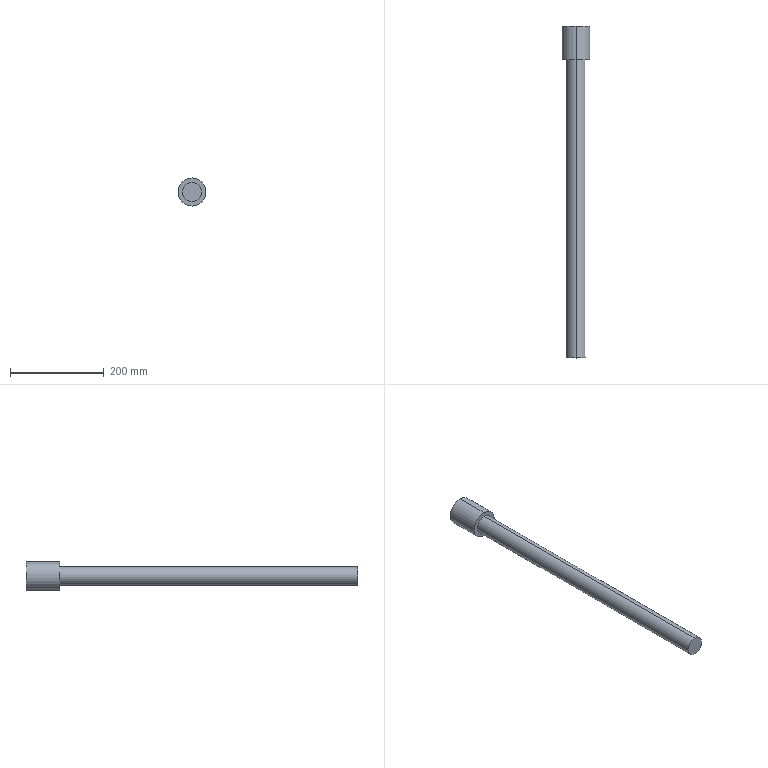Part | SolidWorks | features Revolution 1 | 1 solid | 7 faces | box 60 x 708 x 60 mm | volume 1002796 mm3 | cylinder 4 | plane 3 | commonest cylinder face diameters 40 x2 60 x2
STEP:
#1=CARTESIAN_POINT('',(0.,636.,30.));
#2=VERTEX_POINT('',#1);
#3=CARTESIAN_POINT('',(0.,636.,-30.));
#4=VERTEX_POINT('',#3);
#5=CARTESIAN_POINT('',(0.,636.,0.));
#6=DIRECTION('',(0.,1.,0.));
#7=DIRECTION('',(0.,0.,1.));
#8=AXIS2_PLACEMENT_3D('',#5,#6,#7);
#9=CIRCLE('',#8,30.);
#10=EDGE_CURVE('',#2,#4,#9,.T.);
#11=ORIENTED_EDGE('',*,*,#10,.T.);
#12=CARTESIAN_POINT('',(0.,708.,-30.));
#13=VERTEX_POINT('',#12);
#14=CARTESIAN_POINT('',(0.,0.,-30.));
#15=DIRECTION('',(0.,1.,0.));
#16=VECTOR('',#15,1000.);
#17=LINE('',#14,#16);
#18=EDGE_CURVE('',#4,#13,#17,.T.);
#19=ORIENTED_EDGE('',*,*,#18,.T.);
#20=CARTESIAN_POINT('',(0.,708.,30.));
#21=VERTEX_POINT('',#20);
#22=CARTESIAN_POINT('',(0.,708.,0.));
#23=DIRECTION('',(0.,1.,0.));
#24=DIRECTION('',(0.,0.,1.));
#25=AXIS2_PLACEMENT_3D('',#22,#23,#24);
#26=CIRCLE('',#25,30.);
#27=EDGE_CURVE('',#21,#13,#26,.T.);
#28=ORIENTED_EDGE('',*,*,#27,.F.);
#29=CARTESIAN_POINT('',(0.,0.,30.));
#30=DIRECTION('',(0.,1.,0.));
#31=VECTOR('',#30,1000.);
#32=LINE('',#29,#31);
#33=EDGE_CURVE('',#2,#21,#32,.T.);
#34=ORIENTED_EDGE('',*,*,#33,.F.);
#35=EDGE_LOOP('',(#11,#19,#28,#34));
#36=FACE_OUTER_BOUND('',#35,.T.);
#37=CARTESIAN_POINT('',(0.,0.,0.));
#38=DIRECTION('',(0.,1.,0.));
#39=DIRECTION('',(0.,0.,1.));
#40=AXIS2_PLACEMENT_3D('',#37,#38,#39);
#41=CYLINDRICAL_SURFACE('',#40,30.);
#42=ADVANCED_FACE('',(#36),#41,.T.);
#43=CARTESIAN_POINT('',(0.,0.,20.));
#44=VERTEX_POINT('',#43);
#45=CARTESIAN_POINT('',(0.,0.,-20.));
#46=VERTEX_POINT('',#45);
#47=CARTESIAN_POINT('',(0.,0.,0.));
#48=DIRECTION('',(0.,1.,0.));
#49=DIRECTION('',(0.,0.,1.));
#50=AXIS2_PLACEMENT_3D('',#47,#48,#49);
#51=CIRCLE('',#50,20.);
#52=EDGE_CURVE('',#44,#46,#51,.T.);
#53=ORIENTED_EDGE('',*,*,#52,.T.);
#54=CARTESIAN_POINT('',(0.,636.,-20.));
#55=VERTEX_POINT('',#54);
#56=CARTESIAN_POINT('',(0.,0.,-20.));
#57=DIRECTION('',(0.,1.,0.));
#58=VECTOR('',#57,1000.);
#59=LINE('',#56,#58);
#60=EDGE_CURVE('',#46,#55,#59,.T.);
#61=ORIENTED_EDGE('',*,*,#60,.T.);
#62=CARTESIAN_POINT('',(0.,636.,20.));
#63=VERTEX_POINT('',#62);
#64=CARTESIAN_POINT('',(0.,636.,0.));
#65=DIRECTION('',(0.,1.,0.));
#66=DIRECTION('',(0.,0.,1.));
#67=AXIS2_PLACEMENT_3D('',#64,#65,#66);
#68=CIRCLE('',#67,20.);
#69=EDGE_CURVE('',#63,#55,#68,.T.);
#70=ORIENTED_EDGE('',*,*,#69,.F.);
#71=CARTESIAN_POINT('',(0.,0.,20.));
#72=DIRECTION('',(0.,1.,0.));
#73=VECTOR('',#72,1000.);
#74=LINE('',#71,#73);
#75=EDGE_CURVE('',#44,#63,#74,.T.);
#76=ORIENTED_EDGE('',*,*,#75,.F.);
#77=EDGE_LOOP('',(#53,#61,#70,#76));
#78=FACE_OUTER_BOUND('',#77,.T.);
#79=CARTESIAN_POINT('',(0.,0.,0.));
#80=DIRECTION('',(0.,1.,0.));
#81=DIRECTION('',(0.,0.,1.));
#82=AXIS2_PLACEMENT_3D('',#79,#80,#81);
#83=CYLINDRICAL_SURFACE('',#82,20.);
#84=ADVANCED_FACE('',(#78),#83,.T.);
#85=ORIENTED_EDGE('',*,*,#52,.F.);
#86=CARTESIAN_POINT('',(0.,0.,0.));
#87=DIRECTION('',(0.,1.,0.));
#88=DIRECTION('',(0.,0.,1.));
#89=AXIS2_PLACEMENT_3D('',#86,#87,#88);
#90=CIRCLE('',#89,20.);
#91=EDGE_CURVE('',#46,#44,#90,.T.);
#92=ORIENTED_EDGE('',*,*,#91,.F.);
#93=EDGE_LOOP('',(#85,#92));
#94=FACE_OUTER_BOUND('',#93,.T.);
#95=CARTESIAN_POINT('',(0.,0.,0.));
#96=DIRECTION('',(0.,1.,0.));
#97=DIRECTION('',(0.,0.,1.));
#98=AXIS2_PLACEMENT_3D('',#95,#96,#97);
#99=PLANE('',#98);
#100=ADVANCED_FACE('',(#94),#99,.F.);
#101=ORIENTED_EDGE('',*,*,#60,.F.);
#102=ORIENTED_EDGE('',*,*,#91,.T.);
#103=ORIENTED_EDGE('',*,*,#75,.T.);
#104=CARTESIAN_POINT('',(0.,636.,0.));
#105=DIRECTION('',(0.,1.,0.));
#106=DIRECTION('',(0.,0.,1.));
#107=AXIS2_PLACEMENT_3D('',#104,#105,#106);
#108=CIRCLE('',#107,20.);
#109=EDGE_CURVE('',#55,#63,#108,.T.);
#110=ORIENTED_EDGE('',*,*,#109,.F.);
#111=EDGE_LOOP('',(#101,#102,#103,#110));
#112=FACE_OUTER_BOUND('',#111,.T.);
#113=CARTESIAN_POINT('',(0.,0.,0.));
#114=DIRECTION('',(0.,1.,0.));
#115=DIRECTION('',(0.,0.,1.));
#116=AXIS2_PLACEMENT_3D('',#113,#114,#115);
#117=CYLINDRICAL_SURFACE('',#116,20.);
#118=ADVANCED_FACE('',(#112),#117,.T.);
#119=ORIENTED_EDGE('',*,*,#10,.F.);
#120=CARTESIAN_POINT('',(0.,636.,0.));
#121=DIRECTION('',(0.,1.,0.));
#122=DIRECTION('',(0.,0.,1.));
#123=AXIS2_PLACEMENT_3D('',#120,#121,#122);
#124=CIRCLE('',#123,30.);
#125=EDGE_CURVE('',#4,#2,#124,.T.);
#126=ORIENTED_EDGE('',*,*,#125,.F.);
#127=EDGE_LOOP('',(#119,#126));
#128=FACE_OUTER_BOUND('',#127,.T.);
#129=ORIENTED_EDGE('',*,*,#69,.T.);
#130=ORIENTED_EDGE('',*,*,#109,.T.);
#131=EDGE_LOOP('',(#129,#130));
#132=FACE_BOUND('',#131,.T.);
#133=CARTESIAN_POINT('',(20.,636.,0.));
#134=DIRECTION('',(0.,1.,0.));
#135=DIRECTION('',(0.,0.,1.));
#136=AXIS2_PLACEMENT_3D('',#133,#134,#135);
#137=PLANE('',#136);
#138=ADVANCED_FACE('',(#128,#132),#137,.F.);
#139=ORIENTED_EDGE('',*,*,#18,.F.);
#140=ORIENTED_EDGE('',*,*,#125,.T.);
#141=ORIENTED_EDGE('',*,*,#33,.T.);
#142=CARTESIAN_POINT('',(0.,708.,0.));
#143=DIRECTION('',(0.,1.,0.));
#144=DIRECTION('',(0.,0.,1.));
#145=AXIS2_PLACEMENT_3D('',#142,#143,#144);
#146=CIRCLE('',#145,30.);
#147=EDGE_CURVE('',#13,#21,#146,.T.);
#148=ORIENTED_EDGE('',*,*,#147,.F.);
#149=EDGE_LOOP('',(#139,#140,#141,#148));
#150=FACE_OUTER_BOUND('',#149,.T.);
#151=CARTESIAN_POINT('',(0.,0.,0.));
#152=DIRECTION('',(0.,1.,0.));
#153=DIRECTION('',(0.,0.,1.));
#154=AXIS2_PLACEMENT_3D('',#151,#152,#153);
#155=CYLINDRICAL_SURFACE('',#154,30.);
#156=ADVANCED_FACE('',(#150),#155,.T.);
#157=ORIENTED_EDGE('',*,*,#27,.T.);
#158=ORIENTED_EDGE('',*,*,#147,.T.);
#159=EDGE_LOOP('',(#157,#158));
#160=FACE_OUTER_BOUND('',#159,.T.);
#161=CARTESIAN_POINT('',(30.,708.,0.));
#162=DIRECTION('',(0.,-1.,0.));
#163=DIRECTION('',(0.,0.,-1.));
#164=AXIS2_PLACEMENT_3D('',#161,#162,#163);
#165=PLANE('',#164);
#166=ADVANCED_FACE('',(#160),#165,.F.);
#167=CLOSED_SHELL('',(#42,#84,#100,#118,#138,#156,#166));
#168=MANIFOLD_SOLID_BREP('',#167);
#169=CARTESIAN_POINT('',(0.,0.,0.));
#170=DIRECTION('',(0.,0.,1.));
#171=DIRECTION('',(1.,0.,0.));
#172=AXIS2_PLACEMENT_3D('',#169,#170,#171);
#173=(LENGTH_UNIT()NAMED_UNIT(*)SI_UNIT(.MILLI.,.METRE.));
#174=UNCERTAINTY_MEASURE_WITH_UNIT(LENGTH_MEASURE(0.00001),#173,'','');
#175=(NAMED_UNIT(*)PLANE_ANGLE_UNIT()SI_UNIT($,.RADIAN.));
#176=(NAMED_UNIT(*)SI_UNIT($,.STERADIAN.)SOLID_ANGLE_UNIT());
#177=(GEOMETRIC_REPRESENTATION_CONTEXT(3)GLOBAL_UNCERTAINTY_ASSIGNED_CONTEXT((#174))GLOBAL_UNIT_ASSIGNED_CONTEXT((#173,#175,#176))REPRESENTATION_CONTEXT('',''));
#178=ADVANCED_BREP_SHAPE_REPRESENTATION('',(#168,#172),#177);